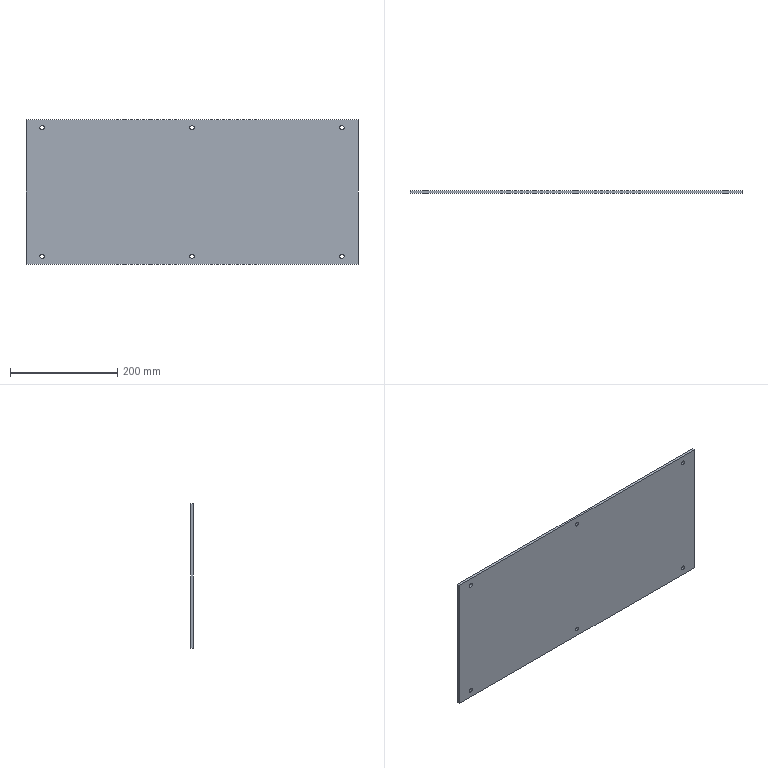Part | STEP file | OP10-003_front cover (R) | 1 solid | 18 faces | box 620 x 5 x 270 mm | volume 835492 mm3 | cylinder 12 | plane 6 | commonest cylinder face diameters 8 x12
STEP:
#1=CARTESIAN_POINT('',(0.,0.,0.));
#2=DIRECTION('',(0.,0.,1.));
#3=DIRECTION('',(1.,0.,0.));
#4=AXIS2_PLACEMENT_3D('',#1,#2,#3);
#5=CARTESIAN_POINT('',(280.,0.,124.));
#6=VERTEX_POINT('',#5);
#7=CARTESIAN_POINT('',(280.,5.,124.));
#8=VERTEX_POINT('',#7);
#9=CARTESIAN_POINT('',(280.,5.,124.));
#10=DIRECTION('',(0.,1.,0.));
#11=VECTOR('',#10,1.);
#12=LINE('',#9,#11);
#13=CARTESIAN_POINT('',(280.,5.,120.));
#14=DIRECTION('',(0.,1.,0.));
#15=DIRECTION('',(0.,0.,1.));
#16=AXIS2_PLACEMENT_3D('',#13,#14,#15);
#17=CYLINDRICAL_SURFACE('',#16,4.);
#18=CARTESIAN_POINT('',(6.283,0.));
#19=DIRECTION('',(0.,1.));
#20=VECTOR('',#19,1.);
#21=LINE('',#18,#20);
#22=(GEOMETRIC_REPRESENTATION_CONTEXT(2)PARAMETRIC_REPRESENTATION_CONTEXT()REPRESENTATION_CONTEXT('',''));
#23=DEFINITIONAL_REPRESENTATION('',(#21),#22);
#24=PCURVE('',#17,#23);
#25=CARTESIAN_POINT('',(280.,5.,120.));
#26=DIRECTION('',(0.,1.,0.));
#27=DIRECTION('',(0.,0.,1.));
#28=AXIS2_PLACEMENT_3D('',#25,#26,#27);
#29=CYLINDRICAL_SURFACE('',#28,4.);
#30=CARTESIAN_POINT('',(0.,0.));
#31=DIRECTION('',(0.,1.));
#32=VECTOR('',#31,1.);
#33=LINE('',#30,#32);
#34=(GEOMETRIC_REPRESENTATION_CONTEXT(2)PARAMETRIC_REPRESENTATION_CONTEXT()REPRESENTATION_CONTEXT('',''));
#35=DEFINITIONAL_REPRESENTATION('',(#33),#34);
#36=PCURVE('',#29,#35);
#37=SURFACE_CURVE('',#12,(#24,#36),.PCURVE_S1.);
#38=EDGE_CURVE('',#6,#8,#37,.T.);
#39=ORIENTED_EDGE('',*,*,#38,.T.);
#40=CARTESIAN_POINT('',(280.,5.,116.));
#41=VERTEX_POINT('',#40);
#42=CARTESIAN_POINT('',(280.,5.,120.));
#43=DIRECTION('',(0.,1.,0.));
#44=DIRECTION('',(0.,0.,1.));
#45=AXIS2_PLACEMENT_3D('',#42,#43,#44);
#46=CIRCLE('',#45,4.);
#47=CARTESIAN_POINT('',(0.,0.));
#48=DIRECTION('',(1.,0.));
#49=VECTOR('',#48,1.);
#50=LINE('',#47,#49);
#51=(GEOMETRIC_REPRESENTATION_CONTEXT(2)PARAMETRIC_REPRESENTATION_CONTEXT()REPRESENTATION_CONTEXT('',''));
#52=DEFINITIONAL_REPRESENTATION('',(#50),#51);
#53=PCURVE('',#17,#52);
#54=CARTESIAN_POINT('',(0.,5.,0.));
#55=DIRECTION('',(0.,-1.,0.));
#56=DIRECTION('',(0.,0.,-1.));
#57=AXIS2_PLACEMENT_3D('',#54,#55,#56);
#58=PLANE('',#57);
#59=CARTESIAN_POINT('',(-124.,280.));
#60=CARTESIAN_POINT('',(-124.,286.928));
#61=CARTESIAN_POINT('',(-118.,283.464));
#62=CARTESIAN_POINT('',(-112.,280.));
#63=CARTESIAN_POINT('',(-118.,276.536));
#64=CARTESIAN_POINT('',(-124.,273.072));
#65=CARTESIAN_POINT('',(-124.,280.));
#66=(BOUNDED_CURVE()B_SPLINE_CURVE(2,(#59,#60,#61,#62,#63,#64,#65),.UNSPECIFIED.,.T.,.F.)B_SPLINE_CURVE_WITH_KNOTS((1,2,2,2,2,1),(-2.094,0.,2.094,4.189,6.283,8.378),.UNSPECIFIED.)CURVE()GEOMETRIC_REPRESENTATION_ITEM()RATIONAL_B_SPLINE_CURVE((1.,0.5,1.,0.5,1.,0.5,1.))REPRESENTATION_ITEM(''));
#67=(GEOMETRIC_REPRESENTATION_CONTEXT(2)PARAMETRIC_REPRESENTATION_CONTEXT()REPRESENTATION_CONTEXT('',''));
#68=DEFINITIONAL_REPRESENTATION('',(#66),#67);
#69=PCURVE('',#58,#68);
#70=SURFACE_CURVE('',#46,(#53,#69),.PCURVE_S1.);
#71=EDGE_CURVE('',#41,#8,#70,.T.);
#72=ORIENTED_EDGE('',*,*,#71,.F.);
#73=CARTESIAN_POINT('',(280.,0.,116.));
#74=VERTEX_POINT('',#73);
#75=CARTESIAN_POINT('',(280.,5.,116.));
#76=DIRECTION('',(0.,1.,0.));
#77=VECTOR('',#76,1.);
#78=LINE('',#75,#77);
#79=CARTESIAN_POINT('',(3.142,0.));
#80=DIRECTION('',(0.,1.));
#81=VECTOR('',#80,1.);
#82=LINE('',#79,#81);
#83=(GEOMETRIC_REPRESENTATION_CONTEXT(2)PARAMETRIC_REPRESENTATION_CONTEXT()REPRESENTATION_CONTEXT('',''));
#84=DEFINITIONAL_REPRESENTATION('',(#82),#83);
#85=PCURVE('',#17,#84);
#86=CARTESIAN_POINT('',(3.142,0.));
#87=DIRECTION('',(0.,1.));
#88=VECTOR('',#87,1.);
#89=LINE('',#86,#88);
#90=(GEOMETRIC_REPRESENTATION_CONTEXT(2)PARAMETRIC_REPRESENTATION_CONTEXT()REPRESENTATION_CONTEXT('',''));
#91=DEFINITIONAL_REPRESENTATION('',(#89),#90);
#92=PCURVE('',#29,#91);
#93=SURFACE_CURVE('',#78,(#85,#92),.PCURVE_S1.);
#94=EDGE_CURVE('',#74,#41,#93,.T.);
#95=ORIENTED_EDGE('',*,*,#94,.F.);
#96=CARTESIAN_POINT('',(280.,0.,120.));
#97=DIRECTION('',(0.,-1.,0.));
#98=DIRECTION('',(0.,0.,-1.));
#99=AXIS2_PLACEMENT_3D('',#96,#97,#98);
#100=CIRCLE('',#99,4.);
#101=CARTESIAN_POINT('',(9.425,-5.));
#102=DIRECTION('',(-1.,0.));
#103=VECTOR('',#102,1.);
#104=LINE('',#101,#103);
#105=(GEOMETRIC_REPRESENTATION_CONTEXT(2)PARAMETRIC_REPRESENTATION_CONTEXT()REPRESENTATION_CONTEXT('',''));
#106=DEFINITIONAL_REPRESENTATION('',(#104),#105);
#107=PCURVE('',#17,#106);
#108=CARTESIAN_POINT('',(0.,0.,0.));
#109=DIRECTION('',(0.,-1.,0.));
#110=DIRECTION('',(0.,0.,-1.));
#111=AXIS2_PLACEMENT_3D('',#108,#109,#110);
#112=PLANE('',#111);
#113=CARTESIAN_POINT('',(-120.,280.));
#114=DIRECTION('',(1.,0.));
#115=AXIS2_PLACEMENT_2D('',#113,#114);
#116=CIRCLE('',#115,4.);
#117=(GEOMETRIC_REPRESENTATION_CONTEXT(2)PARAMETRIC_REPRESENTATION_CONTEXT()REPRESENTATION_CONTEXT('',''));
#118=DEFINITIONAL_REPRESENTATION('',(#116),#117);
#119=PCURVE('',#112,#118);
#120=SURFACE_CURVE('',#100,(#107,#119),.PCURVE_S1.);
#121=EDGE_CURVE('',#6,#74,#120,.T.);
#122=ORIENTED_EDGE('',*,*,#121,.F.);
#123=EDGE_LOOP('',(#39,#72,#95,#122));
#124=FACE_BOUND('',#123,.F.);
#125=ADVANCED_FACE('',(#124),#17,.F.);
#126=CARTESIAN_POINT('',(0.,0.,124.));
#127=VERTEX_POINT('',#126);
#128=CARTESIAN_POINT('',(0.,5.,124.));
#129=VERTEX_POINT('',#128);
#130=CARTESIAN_POINT('',(0.,5.,124.));
#131=DIRECTION('',(0.,1.,0.));
#132=VECTOR('',#131,1.);
#133=LINE('',#130,#132);
#134=CARTESIAN_POINT('',(0.,5.,120.));
#135=DIRECTION('',(0.,1.,0.));
#136=DIRECTION('',(0.,0.,1.));
#137=AXIS2_PLACEMENT_3D('',#134,#135,#136);
#138=CYLINDRICAL_SURFACE('',#137,4.);
#139=CARTESIAN_POINT('',(6.283,0.));
#140=DIRECTION('',(0.,1.));
#141=VECTOR('',#140,1.);
#142=LINE('',#139,#141);
#143=(GEOMETRIC_REPRESENTATION_CONTEXT(2)PARAMETRIC_REPRESENTATION_CONTEXT()REPRESENTATION_CONTEXT('',''));
#144=DEFINITIONAL_REPRESENTATION('',(#142),#143);
#145=PCURVE('',#138,#144);
#146=CARTESIAN_POINT('',(0.,5.,120.));
#147=DIRECTION('',(0.,1.,0.));
#148=DIRECTION('',(0.,0.,1.));
#149=AXIS2_PLACEMENT_3D('',#146,#147,#148);
#150=CYLINDRICAL_SURFACE('',#149,4.);
#151=CARTESIAN_POINT('',(0.,0.));
#152=DIRECTION('',(0.,1.));
#153=VECTOR('',#152,1.);
#154=LINE('',#151,#153);
#155=(GEOMETRIC_REPRESENTATION_CONTEXT(2)PARAMETRIC_REPRESENTATION_CONTEXT()REPRESENTATION_CONTEXT('',''));
#156=DEFINITIONAL_REPRESENTATION('',(#154),#155);
#157=PCURVE('',#150,#156);
#158=SURFACE_CURVE('',#133,(#145,#157),.PCURVE_S1.);
#159=EDGE_CURVE('',#127,#129,#158,.T.);
#160=ORIENTED_EDGE('',*,*,#159,.T.);
#161=CARTESIAN_POINT('',(0.,5.,116.));
#162=VERTEX_POINT('',#161);
#163=CARTESIAN_POINT('',(0.,5.,120.));
#164=DIRECTION('',(0.,1.,0.));
#165=DIRECTION('',(0.,0.,1.));
#166=AXIS2_PLACEMENT_3D('',#163,#164,#165);
#167=CIRCLE('',#166,4.);
#168=CARTESIAN_POINT('',(0.,0.));
#169=DIRECTION('',(1.,0.));
#170=VECTOR('',#169,1.);
#171=LINE('',#168,#170);
#172=(GEOMETRIC_REPRESENTATION_CONTEXT(2)PARAMETRIC_REPRESENTATION_CONTEXT()REPRESENTATION_CONTEXT('',''));
#173=DEFINITIONAL_REPRESENTATION('',(#171),#172);
#174=PCURVE('',#138,#173);
#175=CARTESIAN_POINT('',(-124.,0.));
#176=CARTESIAN_POINT('',(-124.,6.928));
#177=CARTESIAN_POINT('',(-118.,3.464));
#178=CARTESIAN_POINT('',(-112.,0.));
#179=CARTESIAN_POINT('',(-118.,-3.464));
#180=CARTESIAN_POINT('',(-124.,-6.928));
#181=CARTESIAN_POINT('',(-124.,0.));
#182=(BOUNDED_CURVE()B_SPLINE_CURVE(2,(#175,#176,#177,#178,#179,#180,#181),.UNSPECIFIED.,.T.,.F.)B_SPLINE_CURVE_WITH_KNOTS((1,2,2,2,2,1),(-2.094,0.,2.094,4.189,6.283,8.378),.UNSPECIFIED.)CURVE()GEOMETRIC_REPRESENTATION_ITEM()RATIONAL_B_SPLINE_CURVE((1.,0.5,1.,0.5,1.,0.5,1.))REPRESENTATION_ITEM(''));
#183=(GEOMETRIC_REPRESENTATION_CONTEXT(2)PARAMETRIC_REPRESENTATION_CONTEXT()REPRESENTATION_CONTEXT('',''));
#184=DEFINITIONAL_REPRESENTATION('',(#182),#183);
#185=PCURVE('',#58,#184);
#186=SURFACE_CURVE('',#167,(#174,#185),.PCURVE_S1.);
#187=EDGE_CURVE('',#162,#129,#186,.T.);
#188=ORIENTED_EDGE('',*,*,#187,.F.);
#189=CARTESIAN_POINT('',(0.,0.,116.));
#190=VERTEX_POINT('',#189);
#191=CARTESIAN_POINT('',(0.,5.,116.));
#192=DIRECTION('',(0.,1.,0.));
#193=VECTOR('',#192,1.);
#194=LINE('',#191,#193);
#195=CARTESIAN_POINT('',(3.142,0.));
#196=DIRECTION('',(0.,1.));
#197=VECTOR('',#196,1.);
#198=LINE('',#195,#197);
#199=(GEOMETRIC_REPRESENTATION_CONTEXT(2)PARAMETRIC_REPRESENTATION_CONTEXT()REPRESENTATION_CONTEXT('',''));
#200=DEFINITIONAL_REPRESENTATION('',(#198),#199);
#201=PCURVE('',#138,#200);
#202=CARTESIAN_POINT('',(3.142,0.));
#203=DIRECTION('',(0.,1.));
#204=VECTOR('',#203,1.);
#205=LINE('',#202,#204);
#206=(GEOMETRIC_REPRESENTATION_CONTEXT(2)PARAMETRIC_REPRESENTATION_CONTEXT()REPRESENTATION_CONTEXT('',''));
#207=DEFINITIONAL_REPRESENTATION('',(#205),#206);
#208=PCURVE('',#150,#207);
#209=SURFACE_CURVE('',#194,(#201,#208),.PCURVE_S1.);
#210=EDGE_CURVE('',#190,#162,#209,.T.);
#211=ORIENTED_EDGE('',*,*,#210,.F.);
#212=CARTESIAN_POINT('',(0.,0.,120.));
#213=DIRECTION('',(0.,-1.,0.));
#214=DIRECTION('',(0.,0.,-1.));
#215=AXIS2_PLACEMENT_3D('',#212,#213,#214);
#216=CIRCLE('',#215,4.);
#217=CARTESIAN_POINT('',(9.425,-5.));
#218=DIRECTION('',(-1.,0.));
#219=VECTOR('',#218,1.);
#220=LINE('',#217,#219);
#221=(GEOMETRIC_REPRESENTATION_CONTEXT(2)PARAMETRIC_REPRESENTATION_CONTEXT()REPRESENTATION_CONTEXT('',''));
#222=DEFINITIONAL_REPRESENTATION('',(#220),#221);
#223=PCURVE('',#138,#222);
#224=CARTESIAN_POINT('',(-120.,0.));
#225=DIRECTION('',(1.,0.));
#226=AXIS2_PLACEMENT_2D('',#224,#225);
#227=CIRCLE('',#226,4.);
#228=(GEOMETRIC_REPRESENTATION_CONTEXT(2)PARAMETRIC_REPRESENTATION_CONTEXT()REPRESENTATION_CONTEXT('',''));
#229=DEFINITIONAL_REPRESENTATION('',(#227),#228);
#230=PCURVE('',#112,#229);
#231=SURFACE_CURVE('',#216,(#223,#230),.PCURVE_S1.);
#232=EDGE_CURVE('',#127,#190,#231,.T.);
#233=ORIENTED_EDGE('',*,*,#232,.F.);
#234=EDGE_LOOP('',(#160,#188,#211,#233));
#235=FACE_BOUND('',#234,.F.);
#236=ADVANCED_FACE('',(#235),#138,.F.);
#237=CARTESIAN_POINT('',(-280.,0.,124.));
#238=VERTEX_POINT('',#237);
#239=CARTESIAN_POINT('',(-280.,5.,124.));
#240=VERTEX_POINT('',#239);
#241=CARTESIAN_POINT('',(-280.,5.,124.));
#242=DIRECTION('',(0.,1.,0.));
#243=VECTOR('',#242,1.);
#244=LINE('',#241,#243);
#245=CARTESIAN_POINT('',(-280.,5.,120.));
#246=DIRECTION('',(0.,1.,0.));
#247=DIRECTION('',(0.,0.,1.));
#248=AXIS2_PLACEMENT_3D('',#245,#246,#247);
#249=CYLINDRICAL_SURFACE('',#248,4.);
#250=CARTESIAN_POINT('',(6.283,0.));
#251=DIRECTION('',(0.,1.));
#252=VECTOR('',#251,1.);
#253=LINE('',#250,#252);
#254=(GEOMETRIC_REPRESENTATION_CONTEXT(2)PARAMETRIC_REPRESENTATION_CONTEXT()REPRESENTATION_CONTEXT('',''));
#255=DEFINITIONAL_REPRESENTATION('',(#253),#254);
#256=PCURVE('',#249,#255);
#257=CARTESIAN_POINT('',(-280.,5.,120.));
#258=DIRECTION('',(0.,1.,0.));
#259=DIRECTION('',(0.,0.,1.));
#260=AXIS2_PLACEMENT_3D('',#257,#258,#259);
#261=CYLINDRICAL_SURFACE('',#260,4.);
#262=CARTESIAN_POINT('',(0.,0.));
#263=DIRECTION('',(0.,1.));
#264=VECTOR('',#263,1.);
#265=LINE('',#262,#264);
#266=(GEOMETRIC_REPRESENTATION_CONTEXT(2)PARAMETRIC_REPRESENTATION_CONTEXT()REPRESENTATION_CONTEXT('',''));
#267=DEFINITIONAL_REPRESENTATION('',(#265),#266);
#268=PCURVE('',#261,#267);
#269=SURFACE_CURVE('',#244,(#256,#268),.PCURVE_S1.);
#270=EDGE_CURVE('',#238,#240,#269,.T.);
#271=ORIENTED_EDGE('',*,*,#270,.T.);
#272=CARTESIAN_POINT('',(-280.,5.,116.));
#273=VERTEX_POINT('',#272);
#274=CARTESIAN_POINT('',(-280.,5.,120.));
#275=DIRECTION('',(0.,1.,0.));
#276=DIRECTION('',(0.,0.,1.));
#277=AXIS2_PLACEMENT_3D('',#274,#275,#276);
#278=CIRCLE('',#277,4.);
#279=CARTESIAN_POINT('',(0.,0.));
#280=DIRECTION('',(1.,0.));
#281=VECTOR('',#280,1.);
#282=LINE('',#279,#281);
#283=(GEOMETRIC_REPRESENTATION_CONTEXT(2)PARAMETRIC_REPRESENTATION_CONTEXT()REPRESENTATION_CONTEXT('',''));
#284=DEFINITIONAL_REPRESENTATION('',(#282),#283);
#285=PCURVE('',#249,#284);
#286=CARTESIAN_POINT('',(-124.,-280.));
#287=CARTESIAN_POINT('',(-124.,-273.072));
#288=CARTESIAN_POINT('',(-118.,-276.536));
#289=CARTESIAN_POINT('',(-112.,-280.));
#290=CARTESIAN_POINT('',(-118.,-283.464));
#291=CARTESIAN_POINT('',(-124.,-286.928));
#292=CARTESIAN_POINT('',(-124.,-280.));
#293=(BOUNDED_CURVE()B_SPLINE_CURVE(2,(#286,#287,#288,#289,#290,#291,#292),.UNSPECIFIED.,.T.,.F.)B_SPLINE_CURVE_WITH_KNOTS((1,2,2,2,2,1),(-2.094,0.,2.094,4.189,6.283,8.378),.UNSPECIFIED.)CURVE()GEOMETRIC_REPRESENTATION_ITEM()RATIONAL_B_SPLINE_CURVE((1.,0.5,1.,0.5,1.,0.5,1.))REPRESENTATION_ITEM(''));
#294=(GEOMETRIC_REPRESENTATION_CONTEXT(2)PARAMETRIC_REPRESENTATION_CONTEXT()REPRESENTATION_CONTEXT('',''));
#295=DEFINITIONAL_REPRESENTATION('',(#293),#294);
#296=PCURVE('',#58,#295);
#297=SURFACE_CURVE('',#278,(#285,#296),.PCURVE_S1.);
#298=EDGE_CURVE('',#273,#240,#297,.T.);
#299=ORIENTED_EDGE('',*,*,#298,.F.);
#300=CARTESIAN_POINT('',(-280.,0.,116.));
#301=VERTEX_POINT('',#300);
#302=CARTESIAN_POINT('',(-280.,5.,116.));
#303=DIRECTION('',(0.,1.,0.));
#304=VECTOR('',#303,1.);
#305=LINE('',#302,#304);
#306=CARTESIAN_POINT('',(3.142,0.));
#307=DIRECTION('',(0.,1.));
#308=VECTOR('',#307,1.);
#309=LINE('',#306,#308);
#310=(GEOMETRIC_REPRESENTATION_CONTEXT(2)PARAMETRIC_REPRESENTATION_CONTEXT()REPRESENTATION_CONTEXT('',''));
#311=DEFINITIONAL_REPRESENTATION('',(#309),#310);
#312=PCURVE('',#249,#311);
#313=CARTESIAN_POINT('',(3.142,0.));
#314=DIRECTION('',(0.,1.));
#315=VECTOR('',#314,1.);
#316=LINE('',#313,#315);
#317=(GEOMETRIC_REPRESENTATION_CONTEXT(2)PARAMETRIC_REPRESENTATION_CONTEXT()REPRESENTATION_CONTEXT('',''));
#318=DEFINITIONAL_REPRESENTATION('',(#316),#317);
#319=PCURVE('',#261,#318);
#320=SURFACE_CURVE('',#305,(#312,#319),.PCURVE_S1.);
#321=EDGE_CURVE('',#301,#273,#320,.T.);
#322=ORIENTED_EDGE('',*,*,#321,.F.);
#323=CARTESIAN_POINT('',(-280.,0.,120.));
#324=DIRECTION('',(0.,-1.,0.));
#325=DIRECTION('',(0.,0.,-1.));
#326=AXIS2_PLACEMENT_3D('',#323,#324,#325);
#327=CIRCLE('',#326,4.);
#328=CARTESIAN_POINT('',(9.425,-5.));
#329=DIRECTION('',(-1.,0.));
#330=VECTOR('',#329,1.);
#331=LINE('',#328,#330);
#332=(GEOMETRIC_REPRESENTATION_CONTEXT(2)PARAMETRIC_REPRESENTATION_CONTEXT()REPRESENTATION_CONTEXT('',''));
#333=DEFINITIONAL_REPRESENTATION('',(#331),#332);
#334=PCURVE('',#249,#333);
#335=CARTESIAN_POINT('',(-120.,-280.));
#336=DIRECTION('',(1.,0.));
#337=AXIS2_PLACEMENT_2D('',#335,#336);
#338=CIRCLE('',#337,4.);
#339=(GEOMETRIC_REPRESENTATION_CONTEXT(2)PARAMETRIC_REPRESENTATION_CONTEXT()REPRESENTATION_CONTEXT('',''));
#340=DEFINITIONAL_REPRESENTATION('',(#338),#339);
#341=PCURVE('',#112,#340);
#342=SURFACE_CURVE('',#327,(#334,#341),.PCURVE_S1.);
#343=EDGE_CURVE('',#238,#301,#342,.T.);
#344=ORIENTED_EDGE('',*,*,#343,.F.);
#345=EDGE_LOOP('',(#271,#299,#322,#344));
#346=FACE_BOUND('',#345,.F.);
#347=ADVANCED_FACE('',(#346),#249,.F.);
#348=CARTESIAN_POINT('',(280.,0.,-116.));
#349=VERTEX_POINT('',#348);
#350=CARTESIAN_POINT('',(280.,5.,-116.));
#351=VERTEX_POINT('',#350);
#352=CARTESIAN_POINT('',(280.,5.,-116.));
#353=DIRECTION('',(0.,1.,0.));
#354=VECTOR('',#353,1.);
#355=LINE('',#352,#354);
#356=CARTESIAN_POINT('',(280.,5.,-120.));
#357=DIRECTION('',(0.,1.,0.));
#358=DIRECTION('',(0.,0.,1.));
#359=AXIS2_PLACEMENT_3D('',#356,#357,#358);
#360=CYLINDRICAL_SURFACE('',#359,4.);
#361=CARTESIAN_POINT('',(6.283,0.));
#362=DIRECTION('',(0.,1.));
#363=VECTOR('',#362,1.);
#364=LINE('',#361,#363);
#365=(GEOMETRIC_REPRESENTATION_CONTEXT(2)PARAMETRIC_REPRESENTATION_CONTEXT()REPRESENTATION_CONTEXT('',''));
#366=DEFINITIONAL_REPRESENTATION('',(#364),#365);
#367=PCURVE('',#360,#366);
#368=CARTESIAN_POINT('',(280.,5.,-120.));
#369=DIRECTION('',(0.,1.,0.));
#370=DIRECTION('',(0.,0.,1.));
#371=AXIS2_PLACEMENT_3D('',#368,#369,#370);
#372=CYLINDRICAL_SURFACE('',#371,4.);
#373=CARTESIAN_POINT('',(0.,0.));
#374=DIRECTION('',(0.,1.));
#375=VECTOR('',#374,1.);
#376=LINE('',#373,#375);
#377=(GEOMETRIC_REPRESENTATION_CONTEXT(2)PARAMETRIC_REPRESENTATION_CONTEXT()REPRESENTATION_CONTEXT('',''));
#378=DEFINITIONAL_REPRESENTATION('',(#376),#377);
#379=PCURVE('',#372,#378);
#380=SURFACE_CURVE('',#355,(#367,#379),.PCURVE_S1.);
#381=EDGE_CURVE('',#349,#351,#380,.T.);
#382=ORIENTED_EDGE('',*,*,#381,.T.);
#383=CARTESIAN_POINT('',(280.,5.,-124.));
#384=VERTEX_POINT('',#383);
#385=CARTESIAN_POINT('',(280.,5.,-120.));
#386=DIRECTION('',(0.,1.,0.));
#387=DIRECTION('',(0.,0.,1.));
#388=AXIS2_PLACEMENT_3D('',#385,#386,#387);
#389=CIRCLE('',#388,4.);
#390=CARTESIAN_POINT('',(0.,0.));
#391=DIRECTION('',(1.,0.));
#392=VECTOR('',#391,1.);
#393=LINE('',#390,#392);
#394=(GEOMETRIC_REPRESENTATION_CONTEXT(2)PARAMETRIC_REPRESENTATION_CONTEXT()REPRESENTATION_CONTEXT('',''));
#395=DEFINITIONAL_REPRESENTATION('',(#393),#394);
#396=PCURVE('',#360,#395);
#397=CARTESIAN_POINT('',(116.,280.));
#398=CARTESIAN_POINT('',(116.,286.928));
#399=CARTESIAN_POINT('',(122.,283.464));
#400=CARTESIAN_POINT('',(128.,280.));
#401=CARTESIAN_POINT('',(122.,276.536));
#402=CARTESIAN_POINT('',(116.,273.072));
#403=CARTESIAN_POINT('',(116.,280.));
#404=(BOUNDED_CURVE()B_SPLINE_CURVE(2,(#397,#398,#399,#400,#401,#402,#403),.UNSPECIFIED.,.T.,.F.)B_SPLINE_CURVE_WITH_KNOTS((1,2,2,2,2,1),(-2.094,0.,2.094,4.189,6.283,8.378),.UNSPECIFIED.)CURVE()GEOMETRIC_REPRESENTATION_ITEM()RATIONAL_B_SPLINE_CURVE((1.,0.5,1.,0.5,1.,0.5,1.))REPRESENTATION_ITEM(''));
#405=(GEOMETRIC_REPRESENTATION_CONTEXT(2)PARAMETRIC_REPRESENTATION_CONTEXT()REPRESENTATION_CONTEXT('',''));
#406=DEFINITIONAL_REPRESENTATION('',(#404),#405);
#407=PCURVE('',#58,#406);
#408=SURFACE_CURVE('',#389,(#396,#407),.PCURVE_S1.);
#409=EDGE_CURVE('',#384,#351,#408,.T.);
#410=ORIENTED_EDGE('',*,*,#409,.F.);
#411=CARTESIAN_POINT('',(280.,0.,-124.));
#412=VERTEX_POINT('',#411);
#413=CARTESIAN_POINT('',(280.,5.,-124.));
#414=DIRECTION('',(0.,1.,0.));
#415=VECTOR('',#414,1.);
#416=LINE('',#413,#415);
#417=CARTESIAN_POINT('',(3.142,0.));
#418=DIRECTION('',(0.,1.));
#419=VECTOR('',#418,1.);
#420=LINE('',#417,#419);
#421=(GEOMETRIC_REPRESENTATION_CONTEXT(2)PARAMETRIC_REPRESENTATION_CONTEXT()REPRESENTATION_CONTEXT('',''));
#422=DEFINITIONAL_REPRESENTATION('',(#420),#421);
#423=PCURVE('',#360,#422);
#424=CARTESIAN_POINT('',(3.142,0.));
#425=DIRECTION('',(0.,1.));
#426=VECTOR('',#425,1.);
#427=LINE('',#424,#426);
#428=(GEOMETRIC_REPRESENTATION_CONTEXT(2)PARAMETRIC_REPRESENTATION_CONTEXT()REPRESENTATION_CONTEXT('',''));
#429=DEFINITIONAL_REPRESENTATION('',(#427),#428);
#430=PCURVE('',#372,#429);
#431=SURFACE_CURVE('',#416,(#423,#430),.PCURVE_S1.);
#432=EDGE_CURVE('',#412,#384,#431,.T.);
#433=ORIENTED_EDGE('',*,*,#432,.F.);
#434=CARTESIAN_POINT('',(280.,0.,-120.));
#435=DIRECTION('',(0.,-1.,0.));
#436=DIRECTION('',(0.,0.,-1.));
#437=AXIS2_PLACEMENT_3D('',#434,#435,#436);
#438=CIRCLE('',#437,4.);
#439=CARTESIAN_POINT('',(9.425,-5.));
#440=DIRECTION('',(-1.,0.));
#441=VECTOR('',#440,1.);
#442=LINE('',#439,#441);
#443=(GEOMETRIC_REPRESENTATION_CONTEXT(2)PARAMETRIC_REPRESENTATION_CONTEXT()REPRESENTATION_CONTEXT('',''));
#444=DEFINITIONAL_REPRESENTATION('',(#442),#443);
#445=PCURVE('',#360,#444);
#446=CARTESIAN_POINT('',(120.,280.));
#447=DIRECTION('',(1.,0.));
#448=AXIS2_PLACEMENT_2D('',#446,#447);
#449=CIRCLE('',#448,4.);
#450=(GEOMETRIC_REPRESENTATION_CONTEXT(2)PARAMETRIC_REPRESENTATION_CONTEXT()REPRESENTATION_CONTEXT('',''));
#451=DEFINITIONAL_REPRESENTATION('',(#449),#450);
#452=PCURVE('',#112,#451);
#453=SURFACE_CURVE('',#438,(#445,#452),.PCURVE_S1.);
#454=EDGE_CURVE('',#349,#412,#453,.T.);
#455=ORIENTED_EDGE('',*,*,#454,.F.);
#456=EDGE_LOOP('',(#382,#410,#433,#455));
#457=FACE_BOUND('',#456,.F.);
#458=ADVANCED_FACE('',(#457),#360,.F.);
#459=CARTESIAN_POINT('',(0.,0.,-116.));
#460=VERTEX_POINT('',#459);
#461=CARTESIAN_POINT('',(0.,5.,-116.));
#462=VERTEX_POINT('',#461);
#463=CARTESIAN_POINT('',(0.,5.,-116.));
#464=DIRECTION('',(0.,1.,0.));
#465=VECTOR('',#464,1.);
#466=LINE('',#463,#465);
#467=CARTESIAN_POINT('',(0.,5.,-120.));
#468=DIRECTION('',(0.,1.,0.));
#469=DIRECTION('',(0.,0.,1.));
#470=AXIS2_PLACEMENT_3D('',#467,#468,#469);
#471=CYLINDRICAL_SURFACE('',#470,4.);
#472=CARTESIAN_POINT('',(6.283,0.));
#473=DIRECTION('',(0.,1.));
#474=VECTOR('',#473,1.);
#475=LINE('',#472,#474);
#476=(GEOMETRIC_REPRESENTATION_CONTEXT(2)PARAMETRIC_REPRESENTATION_CONTEXT()REPRESENTATION_CONTEXT('',''));
#477=DEFINITIONAL_REPRESENTATION('',(#475),#476);
#478=PCURVE('',#471,#477);
#479=CARTESIAN_POINT('',(0.,5.,-120.));
#480=DIRECTION('',(0.,1.,0.));
#481=DIRECTION('',(0.,0.,1.));
#482=AXIS2_PLACEMENT_3D('',#479,#480,#481);
#483=CYLINDRICAL_SURFACE('',#482,4.);
#484=CARTESIAN_POINT('',(0.,0.));
#485=DIRECTION('',(0.,1.));
#486=VECTOR('',#485,1.);
#487=LINE('',#484,#486);
#488=(GEOMETRIC_REPRESENTATION_CONTEXT(2)PARAMETRIC_REPRESENTATION_CONTEXT()REPRESENTATION_CONTEXT('',''));
#489=DEFINITIONAL_REPRESENTATION('',(#487),#488);
#490=PCURVE('',#483,#489);
#491=SURFACE_CURVE('',#466,(#478,#490),.PCURVE_S1.);
#492=EDGE_CURVE('',#460,#462,#491,.T.);
#493=ORIENTED_EDGE('',*,*,#492,.T.);
#494=CARTESIAN_POINT('',(0.,5.,-124.));
#495=VERTEX_POINT('',#494);
#496=CARTESIAN_POINT('',(0.,5.,-120.));
#497=DIRECTION('',(0.,1.,0.));
#498=DIRECTION('',(0.,0.,1.));
#499=AXIS2_PLACEMENT_3D('',#496,#497,#498);
#500=CIRCLE('',#499,4.);
#501=CARTESIAN_POINT('',(0.,0.));
#502=DIRECTION('',(1.,0.));
#503=VECTOR('',#502,1.);
#504=LINE('',#501,#503);
#505=(GEOMETRIC_REPRESENTATION_CONTEXT(2)PARAMETRIC_REPRESENTATION_CONTEXT()REPRESENTATION_CONTEXT('',''));
#506=DEFINITIONAL_REPRESENTATION('',(#504),#505);
#507=PCURVE('',#471,#506);
#508=CARTESIAN_POINT('',(116.,0.));
#509=CARTESIAN_POINT('',(116.,6.928));
#510=CARTESIAN_POINT('',(122.,3.464));
#511=CARTESIAN_POINT('',(128.,0.));
#512=CARTESIAN_POINT('',(122.,-3.464));
#513=CARTESIAN_POINT('',(116.,-6.928));
#514=CARTESIAN_POINT('',(116.,0.));
#515=(BOUNDED_CURVE()B_SPLINE_CURVE(2,(#508,#509,#510,#511,#512,#513,#514),.UNSPECIFIED.,.T.,.F.)B_SPLINE_CURVE_WITH_KNOTS((1,2,2,2,2,1),(-2.094,0.,2.094,4.189,6.283,8.378),.UNSPECIFIED.)CURVE()GEOMETRIC_REPRESENTATION_ITEM()RATIONAL_B_SPLINE_CURVE((1.,0.5,1.,0.5,1.,0.5,1.))REPRESENTATION_ITEM(''));
#516=(GEOMETRIC_REPRESENTATION_CONTEXT(2)PARAMETRIC_REPRESENTATION_CONTEXT()REPRESENTATION_CONTEXT('',''));
#517=DEFINITIONAL_REPRESENTATION('',(#515),#516);
#518=PCURVE('',#58,#517);
#519=SURFACE_CURVE('',#500,(#507,#518),.PCURVE_S1.);
#520=EDGE_CURVE('',#495,#462,#519,.T.);
#521=ORIENTED_EDGE('',*,*,#520,.F.);
#522=CARTESIAN_POINT('',(0.,0.,-124.));
#523=VERTEX_POINT('',#522);
#524=CARTESIAN_POINT('',(0.,5.,-124.));
#525=DIRECTION('',(0.,1.,0.));
#526=VECTOR('',#525,1.);
#527=LINE('',#524,#526);
#528=CARTESIAN_POINT('',(3.142,0.));
#529=DIRECTION('',(0.,1.));
#530=VECTOR('',#529,1.);
#531=LINE('',#528,#530);
#532=(GEOMETRIC_REPRESENTATION_CONTEXT(2)PARAMETRIC_REPRESENTATION_CONTEXT()REPRESENTATION_CONTEXT('',''));
#533=DEFINITIONAL_REPRESENTATION('',(#531),#532);
#534=PCURVE('',#471,#533);
#535=CARTESIAN_POINT('',(3.142,0.));
#536=DIRECTION('',(0.,1.));
#537=VECTOR('',#536,1.);
#538=LINE('',#535,#537);
#539=(GEOMETRIC_REPRESENTATION_CONTEXT(2)PARAMETRIC_REPRESENTATION_CONTEXT()REPRESENTATION_CONTEXT('',''));
#540=DEFINITIONAL_REPRESENTATION('',(#538),#539);
#541=PCURVE('',#483,#540);
#542=SURFACE_CURVE('',#527,(#534,#541),.PCURVE_S1.);
#543=EDGE_CURVE('',#523,#495,#542,.T.);
#544=ORIENTED_EDGE('',*,*,#543,.F.);
#545=CARTESIAN_POINT('',(0.,0.,-120.));
#546=DIRECTION('',(0.,-1.,0.));
#547=DIRECTION('',(0.,0.,-1.));
#548=AXIS2_PLACEMENT_3D('',#545,#546,#547);
#549=CIRCLE('',#548,4.);
#550=CARTESIAN_POINT('',(9.425,-5.));
#551=DIRECTION('',(-1.,0.));
#552=VECTOR('',#551,1.);
#553=LINE('',#550,#552);
#554=(GEOMETRIC_REPRESENTATION_CONTEXT(2)PARAMETRIC_REPRESENTATION_CONTEXT()REPRESENTATION_CONTEXT('',''));
#555=DEFINITIONAL_REPRESENTATION('',(#553),#554);
#556=PCURVE('',#471,#555);
#557=CARTESIAN_POINT('',(120.,0.));
#558=DIRECTION('',(1.,0.));
#559=AXIS2_PLACEMENT_2D('',#557,#558);
#560=CIRCLE('',#559,4.);
#561=(GEOMETRIC_REPRESENTATION_CONTEXT(2)PARAMETRIC_REPRESENTATION_CONTEXT()REPRESENTATION_CONTEXT('',''));
#562=DEFINITIONAL_REPRESENTATION('',(#560),#561);
#563=PCURVE('',#112,#562);
#564=SURFACE_CURVE('',#549,(#556,#563),.PCURVE_S1.);
#565=EDGE_CURVE('',#460,#523,#564,.T.);
#566=ORIENTED_EDGE('',*,*,#565,.F.);
#567=EDGE_LOOP('',(#493,#521,#544,#566));
#568=FACE_BOUND('',#567,.F.);
#569=ADVANCED_FACE('',(#568),#471,.F.);
#570=CARTESIAN_POINT('',(-280.,0.,-116.));
#571=VERTEX_POINT('',#570);
#572=CARTESIAN_POINT('',(-280.,5.,-116.));
#573=VERTEX_POINT('',#572);
#574=CARTESIAN_POINT('',(-280.,5.,-116.));
#575=DIRECTION('',(0.,1.,0.));
#576=VECTOR('',#575,1.);
#577=LINE('',#574,#576);
#578=CARTESIAN_POINT('',(-280.,5.,-120.));
#579=DIRECTION('',(0.,1.,0.));
#580=DIRECTION('',(0.,0.,1.));
#581=AXIS2_PLACEMENT_3D('',#578,#579,#580);
#582=CYLINDRICAL_SURFACE('',#581,4.);
#583=CARTESIAN_POINT('',(6.283,0.));
#584=DIRECTION('',(0.,1.));
#585=VECTOR('',#584,1.);
#586=LINE('',#583,#585);
#587=(GEOMETRIC_REPRESENTATION_CONTEXT(2)PARAMETRIC_REPRESENTATION_CONTEXT()REPRESENTATION_CONTEXT('',''));
#588=DEFINITIONAL_REPRESENTATION('',(#586),#587);
#589=PCURVE('',#582,#588);
#590=CARTESIAN_POINT('',(-280.,5.,-120.));
#591=DIRECTION('',(0.,1.,0.));
#592=DIRECTION('',(0.,0.,1.));
#593=AXIS2_PLACEMENT_3D('',#590,#591,#592);
#594=CYLINDRICAL_SURFACE('',#593,4.);
#595=CARTESIAN_POINT('',(0.,0.));
#596=DIRECTION('',(0.,1.));
#597=VECTOR('',#596,1.);
#598=LINE('',#595,#597);
#599=(GEOMETRIC_REPRESENTATION_CONTEXT(2)PARAMETRIC_REPRESENTATION_CONTEXT()REPRESENTATION_CONTEXT('',''));
#600=DEFINITIONAL_REPRESENTATION('',(#598),#599);
#601=PCURVE('',#594,#600);
#602=SURFACE_CURVE('',#577,(#589,#601),.PCURVE_S1.);
#603=EDGE_CURVE('',#571,#573,#602,.T.);
#604=ORIENTED_EDGE('',*,*,#603,.T.);
#605=CARTESIAN_POINT('',(-280.,5.,-124.));
#606=VERTEX_POINT('',#605);
#607=CARTESIAN_POINT('',(-280.,5.,-120.));
#608=DIRECTION('',(0.,1.,0.));
#609=DIRECTION('',(0.,0.,1.));
#610=AXIS2_PLACEMENT_3D('',#607,#608,#609);
#611=CIRCLE('',#610,4.);
#612=CARTESIAN_POINT('',(0.,0.));
#613=DIRECTION('',(1.,0.));
#614=VECTOR('',#613,1.);
#615=LINE('',#612,#614);
#616=(GEOMETRIC_REPRESENTATION_CONTEXT(2)PARAMETRIC_REPRESENTATION_CONTEXT()REPRESENTATION_CONTEXT('',''));
#617=DEFINITIONAL_REPRESENTATION('',(#615),#616);
#618=PCURVE('',#582,#617);
#619=CARTESIAN_POINT('',(116.,-280.));
#620=CARTESIAN_POINT('',(116.,-273.072));
#621=CARTESIAN_POINT('',(122.,-276.536));
#622=CARTESIAN_POINT('',(128.,-280.));
#623=CARTESIAN_POINT('',(122.,-283.464));
#624=CARTESIAN_POINT('',(116.,-286.928));
#625=CARTESIAN_POINT('',(116.,-280.));
#626=(BOUNDED_CURVE()B_SPLINE_CURVE(2,(#619,#620,#621,#622,#623,#624,#625),.UNSPECIFIED.,.T.,.F.)B_SPLINE_CURVE_WITH_KNOTS((1,2,2,2,2,1),(-2.094,0.,2.094,4.189,6.283,8.378),.UNSPECIFIED.)CURVE()GEOMETRIC_REPRESENTATION_ITEM()RATIONAL_B_SPLINE_CURVE((1.,0.5,1.,0.5,1.,0.5,1.))REPRESENTATION_ITEM(''));
#627=(GEOMETRIC_REPRESENTATION_CONTEXT(2)PARAMETRIC_REPRESENTATION_CONTEXT()REPRESENTATION_CONTEXT('',''));
#628=DEFINITIONAL_REPRESENTATION('',(#626),#627);
#629=PCURVE('',#58,#628);
#630=SURFACE_CURVE('',#611,(#618,#629),.PCURVE_S1.);
#631=EDGE_CURVE('',#606,#573,#630,.T.);
#632=ORIENTED_EDGE('',*,*,#631,.F.);
#633=CARTESIAN_POINT('',(-280.,0.,-124.));
#634=VERTEX_POINT('',#633);
#635=CARTESIAN_POINT('',(-280.,5.,-124.));
#636=DIRECTION('',(0.,1.,0.));
#637=VECTOR('',#636,1.);
#638=LINE('',#635,#637);
#639=CARTESIAN_POINT('',(3.142,0.));
#640=DIRECTION('',(0.,1.));
#641=VECTOR('',#640,1.);
#642=LINE('',#639,#641);
#643=(GEOMETRIC_REPRESENTATION_CONTEXT(2)PARAMETRIC_REPRESENTATION_CONTEXT()REPRESENTATION_CONTEXT('',''));
#644=DEFINITIONAL_REPRESENTATION('',(#642),#643);
#645=PCURVE('',#582,#644);
#646=CARTESIAN_POINT('',(3.142,0.));
#647=DIRECTION('',(0.,1.));
#648=VECTOR('',#647,1.);
#649=LINE('',#646,#648);
#650=(GEOMETRIC_REPRESENTATION_CONTEXT(2)PARAMETRIC_REPRESENTATION_CONTEXT()REPRESENTATION_CONTEXT('',''));
#651=DEFINITIONAL_REPRESENTATION('',(#649),#650);
#652=PCURVE('',#594,#651);
#653=SURFACE_CURVE('',#638,(#645,#652),.PCURVE_S1.);
#654=EDGE_CURVE('',#634,#606,#653,.T.);
#655=ORIENTED_EDGE('',*,*,#654,.F.);
#656=CARTESIAN_POINT('',(-280.,0.,-120.));
#657=DIRECTION('',(0.,-1.,0.));
#658=DIRECTION('',(0.,0.,-1.));
#659=AXIS2_PLACEMENT_3D('',#656,#657,#658);
#660=CIRCLE('',#659,4.);
#661=CARTESIAN_POINT('',(9.425,-5.));
#662=DIRECTION('',(-1.,0.));
#663=VECTOR('',#662,1.);
#664=LINE('',#661,#663);
#665=(GEOMETRIC_REPRESENTATION_CONTEXT(2)PARAMETRIC_REPRESENTATION_CONTEXT()REPRESENTATION_CONTEXT('',''));
#666=DEFINITIONAL_REPRESENTATION('',(#664),#665);
#667=PCURVE('',#582,#666);
#668=CARTESIAN_POINT('',(120.,-280.));
#669=DIRECTION('',(1.,0.));
#670=AXIS2_PLACEMENT_2D('',#668,#669);
#671=CIRCLE('',#670,4.);
#672=(GEOMETRIC_REPRESENTATION_CONTEXT(2)PARAMETRIC_REPRESENTATION_CONTEXT()REPRESENTATION_CONTEXT('',''));
#673=DEFINITIONAL_REPRESENTATION('',(#671),#672);
#674=PCURVE('',#112,#673);
#675=SURFACE_CURVE('',#660,(#667,#674),.PCURVE_S1.);
#676=EDGE_CURVE('',#571,#634,#675,.T.);
#677=ORIENTED_EDGE('',*,*,#676,.F.);
#678=EDGE_LOOP('',(#604,#632,#655,#677));
#679=FACE_BOUND('',#678,.F.);
#680=ADVANCED_FACE('',(#679),#582,.F.);
#681=CARTESIAN_POINT('',(310.,0.,135.));
#682=VERTEX_POINT('',#681);
#683=CARTESIAN_POINT('',(310.,0.,-135.));
#684=VERTEX_POINT('',#683);
#685=CARTESIAN_POINT('',(310.,0.,135.));
#686=DIRECTION('',(0.,0.,-1.));
#687=VECTOR('',#686,1.);
#688=LINE('',#685,#687);
#689=CARTESIAN_POINT('',(310.,5.,135.));
#690=DIRECTION('',(-1.,0.,0.));
#691=DIRECTION('',(0.,0.,1.));
#692=AXIS2_PLACEMENT_3D('',#689,#690,#691);
#693=PLANE('',#692);
#694=CARTESIAN_POINT('',(0.,-5.));
#695=DIRECTION('',(-1.,0.));
#696=VECTOR('',#695,1.);
#697=LINE('',#694,#696);
#698=(GEOMETRIC_REPRESENTATION_CONTEXT(2)PARAMETRIC_REPRESENTATION_CONTEXT()REPRESENTATION_CONTEXT('',''));
#699=DEFINITIONAL_REPRESENTATION('',(#697),#698);
#700=PCURVE('',#693,#699);
#701=CARTESIAN_POINT('',(-135.,310.));
#702=DIRECTION('',(1.,0.));
#703=VECTOR('',#702,1.);
#704=LINE('',#701,#703);
#705=(GEOMETRIC_REPRESENTATION_CONTEXT(2)PARAMETRIC_REPRESENTATION_CONTEXT()REPRESENTATION_CONTEXT('',''));
#706=DEFINITIONAL_REPRESENTATION('',(#704),#705);
#707=PCURVE('',#112,#706);
#708=SURFACE_CURVE('',#688,(#700,#707),.PCURVE_S1.);
#709=EDGE_CURVE('',#682,#684,#708,.T.);
#710=ORIENTED_EDGE('',*,*,#709,.T.);
#711=CARTESIAN_POINT('',(310.,5.,-135.));
#712=VERTEX_POINT('',#711);
#713=CARTESIAN_POINT('',(310.,5.,-135.));
#714=DIRECTION('',(0.,-1.,0.));
#715=VECTOR('',#714,1.);
#716=LINE('',#713,#715);
#717=CARTESIAN_POINT('',(-270.,0.));
#718=DIRECTION('',(0.,-1.));
#719=VECTOR('',#718,1.);
#720=LINE('',#717,#719);
#721=(GEOMETRIC_REPRESENTATION_CONTEXT(2)PARAMETRIC_REPRESENTATION_CONTEXT()REPRESENTATION_CONTEXT('',''));
#722=DEFINITIONAL_REPRESENTATION('',(#720),#721);
#723=PCURVE('',#693,#722);
#724=CARTESIAN_POINT('',(-310.,5.,-135.));
#725=DIRECTION('',(0.,0.,1.));
#726=DIRECTION('',(1.,0.,0.));
#727=AXIS2_PLACEMENT_3D('',#724,#725,#726);
#728=PLANE('',#727);
#729=CARTESIAN_POINT('',(620.,0.));
#730=DIRECTION('',(0.,-1.));
#731=VECTOR('',#730,1.);
#732=LINE('',#729,#731);
#733=(GEOMETRIC_REPRESENTATION_CONTEXT(2)PARAMETRIC_REPRESENTATION_CONTEXT()REPRESENTATION_CONTEXT('',''));
#734=DEFINITIONAL_REPRESENTATION('',(#732),#733);
#735=PCURVE('',#728,#734);
#736=SURFACE_CURVE('',#716,(#723,#735),.PCURVE_S1.);
#737=EDGE_CURVE('',#712,#684,#736,.T.);
#738=ORIENTED_EDGE('',*,*,#737,.F.);
#739=CARTESIAN_POINT('',(310.,5.,135.));
#740=VERTEX_POINT('',#739);
#741=CARTESIAN_POINT('',(310.,5.,135.));
#742=DIRECTION('',(0.,0.,-1.));
#743=VECTOR('',#742,1.);
#744=LINE('',#741,#743);
#745=CARTESIAN_POINT('',(0.,0.));
#746=DIRECTION('',(-1.,0.));
#747=VECTOR('',#746,1.);
#748=LINE('',#745,#747);
#749=(GEOMETRIC_REPRESENTATION_CONTEXT(2)PARAMETRIC_REPRESENTATION_CONTEXT()REPRESENTATION_CONTEXT('',''));
#750=DEFINITIONAL_REPRESENTATION('',(#748),#749);
#751=PCURVE('',#693,#750);
#752=CARTESIAN_POINT('',(-135.,310.));
#753=DIRECTION('',(1.,0.));
#754=VECTOR('',#753,1.);
#755=LINE('',#752,#754);
#756=(GEOMETRIC_REPRESENTATION_CONTEXT(2)PARAMETRIC_REPRESENTATION_CONTEXT()REPRESENTATION_CONTEXT('',''));
#757=DEFINITIONAL_REPRESENTATION('',(#755),#756);
#758=PCURVE('',#58,#757);
#759=SURFACE_CURVE('',#744,(#751,#758),.PCURVE_S1.);
#760=EDGE_CURVE('',#740,#712,#759,.T.);
#761=ORIENTED_EDGE('',*,*,#760,.F.);
#762=CARTESIAN_POINT('',(310.,5.,135.));
#763=DIRECTION('',(0.,-1.,0.));
#764=VECTOR('',#763,1.);
#765=LINE('',#762,#764);
#766=CARTESIAN_POINT('',(0.,0.));
#767=DIRECTION('',(0.,-1.));
#768=VECTOR('',#767,1.);
#769=LINE('',#766,#768);
#770=(GEOMETRIC_REPRESENTATION_CONTEXT(2)PARAMETRIC_REPRESENTATION_CONTEXT()REPRESENTATION_CONTEXT('',''));
#771=DEFINITIONAL_REPRESENTATION('',(#769),#770);
#772=PCURVE('',#693,#771);
#773=CARTESIAN_POINT('',(-310.,5.,135.));
#774=DIRECTION('',(0.,0.,-1.));
#775=DIRECTION('',(-1.,0.,0.));
#776=AXIS2_PLACEMENT_3D('',#773,#774,#775);
#777=PLANE('',#776);
#778=CARTESIAN_POINT('',(-620.,0.));
#779=DIRECTION('',(0.,-1.));
#780=VECTOR('',#779,1.);
#781=LINE('',#778,#780);
#782=(GEOMETRIC_REPRESENTATION_CONTEXT(2)PARAMETRIC_REPRESENTATION_CONTEXT()REPRESENTATION_CONTEXT('',''));
#783=DEFINITIONAL_REPRESENTATION('',(#781),#782);
#784=PCURVE('',#777,#783);
#785=SURFACE_CURVE('',#765,(#772,#784),.PCURVE_S1.);
#786=EDGE_CURVE('',#740,#682,#785,.T.);
#787=ORIENTED_EDGE('',*,*,#786,.T.);
#788=EDGE_LOOP('',(#710,#738,#761,#787));
#789=FACE_BOUND('',#788,.T.);
#790=ADVANCED_FACE('',(#789),#693,.F.);
#791=CARTESIAN_POINT('',(-310.,0.,-135.));
#792=VERTEX_POINT('',#791);
#793=CARTESIAN_POINT('',(-310.,0.,-135.));
#794=DIRECTION('',(-1.,0.,0.));
#795=VECTOR('',#794,1.);
#796=LINE('',#793,#795);
#797=CARTESIAN_POINT('',(0.,-5.));
#798=DIRECTION('',(-1.,0.));
#799=VECTOR('',#798,1.);
#800=LINE('',#797,#799);
#801=(GEOMETRIC_REPRESENTATION_CONTEXT(2)PARAMETRIC_REPRESENTATION_CONTEXT()REPRESENTATION_CONTEXT('',''));
#802=DEFINITIONAL_REPRESENTATION('',(#800),#801);
#803=PCURVE('',#728,#802);
#804=CARTESIAN_POINT('',(135.,-310.));
#805=DIRECTION('',(0.,-1.));
#806=VECTOR('',#805,1.);
#807=LINE('',#804,#806);
#808=(GEOMETRIC_REPRESENTATION_CONTEXT(2)PARAMETRIC_REPRESENTATION_CONTEXT()REPRESENTATION_CONTEXT('',''));
#809=DEFINITIONAL_REPRESENTATION('',(#807),#808);
#810=PCURVE('',#112,#809);
#811=SURFACE_CURVE('',#796,(#803,#810),.PCURVE_S1.);
#812=EDGE_CURVE('',#684,#792,#811,.T.);
#813=ORIENTED_EDGE('',*,*,#812,.T.);
#814=CARTESIAN_POINT('',(-310.,5.,-135.));
#815=VERTEX_POINT('',#814);
#816=CARTESIAN_POINT('',(-310.,5.,-135.));
#817=DIRECTION('',(0.,-1.,0.));
#818=VECTOR('',#817,1.);
#819=LINE('',#816,#818);
#820=CARTESIAN_POINT('',(0.,0.));
#821=DIRECTION('',(0.,-1.));
#822=VECTOR('',#821,1.);
#823=LINE('',#820,#822);
#824=(GEOMETRIC_REPRESENTATION_CONTEXT(2)PARAMETRIC_REPRESENTATION_CONTEXT()REPRESENTATION_CONTEXT('',''));
#825=DEFINITIONAL_REPRESENTATION('',(#823),#824);
#826=PCURVE('',#728,#825);
#827=CARTESIAN_POINT('',(-310.,5.,135.));
#828=DIRECTION('',(1.,0.,0.));
#829=DIRECTION('',(0.,0.,-1.));
#830=AXIS2_PLACEMENT_3D('',#827,#828,#829);
#831=PLANE('',#830);
#832=CARTESIAN_POINT('',(270.,0.));
#833=DIRECTION('',(0.,-1.));
#834=VECTOR('',#833,1.);
#835=LINE('',#832,#834);
#836=(GEOMETRIC_REPRESENTATION_CONTEXT(2)PARAMETRIC_REPRESENTATION_CONTEXT()REPRESENTATION_CONTEXT('',''));
#837=DEFINITIONAL_REPRESENTATION('',(#835),#836);
#838=PCURVE('',#831,#837);
#839=SURFACE_CURVE('',#819,(#826,#838),.PCURVE_S1.);
#840=EDGE_CURVE('',#815,#792,#839,.T.);
#841=ORIENTED_EDGE('',*,*,#840,.F.);
#842=CARTESIAN_POINT('',(-310.,5.,-135.));
#843=DIRECTION('',(-1.,0.,0.));
#844=VECTOR('',#843,1.);
#845=LINE('',#842,#844);
#846=CARTESIAN_POINT('',(0.,0.));
#847=DIRECTION('',(-1.,0.));
#848=VECTOR('',#847,1.);
#849=LINE('',#846,#848);
#850=(GEOMETRIC_REPRESENTATION_CONTEXT(2)PARAMETRIC_REPRESENTATION_CONTEXT()REPRESENTATION_CONTEXT('',''));
#851=DEFINITIONAL_REPRESENTATION('',(#849),#850);
#852=PCURVE('',#728,#851);
#853=CARTESIAN_POINT('',(135.,-310.));
#854=DIRECTION('',(0.,-1.));
#855=VECTOR('',#854,1.);
#856=LINE('',#853,#855);
#857=(GEOMETRIC_REPRESENTATION_CONTEXT(2)PARAMETRIC_REPRESENTATION_CONTEXT()REPRESENTATION_CONTEXT('',''));
#858=DEFINITIONAL_REPRESENTATION('',(#856),#857);
#859=PCURVE('',#58,#858);
#860=SURFACE_CURVE('',#845,(#852,#859),.PCURVE_S1.);
#861=EDGE_CURVE('',#712,#815,#860,.T.);
#862=ORIENTED_EDGE('',*,*,#861,.F.);
#863=ORIENTED_EDGE('',*,*,#737,.T.);
#864=EDGE_LOOP('',(#813,#841,#862,#863));
#865=FACE_BOUND('',#864,.T.);
#866=ADVANCED_FACE('',(#865),#728,.F.);
#867=CARTESIAN_POINT('',(-310.,0.,135.));
#868=VERTEX_POINT('',#867);
#869=CARTESIAN_POINT('',(-310.,0.,135.));
#870=DIRECTION('',(0.,0.,1.));
#871=VECTOR('',#870,1.);
#872=LINE('',#869,#871);
#873=CARTESIAN_POINT('',(0.,-5.));
#874=DIRECTION('',(-1.,0.));
#875=VECTOR('',#874,1.);
#876=LINE('',#873,#875);
#877=(GEOMETRIC_REPRESENTATION_CONTEXT(2)PARAMETRIC_REPRESENTATION_CONTEXT()REPRESENTATION_CONTEXT('',''));
#878=DEFINITIONAL_REPRESENTATION('',(#876),#877);
#879=PCURVE('',#831,#878);
#880=CARTESIAN_POINT('',(-135.,-310.));
#881=DIRECTION('',(-1.,0.));
#882=VECTOR('',#881,1.);
#883=LINE('',#880,#882);
#884=(GEOMETRIC_REPRESENTATION_CONTEXT(2)PARAMETRIC_REPRESENTATION_CONTEXT()REPRESENTATION_CONTEXT('',''));
#885=DEFINITIONAL_REPRESENTATION('',(#883),#884);
#886=PCURVE('',#112,#885);
#887=SURFACE_CURVE('',#872,(#879,#886),.PCURVE_S1.);
#888=EDGE_CURVE('',#792,#868,#887,.T.);
#889=ORIENTED_EDGE('',*,*,#888,.T.);
#890=CARTESIAN_POINT('',(-310.,5.,135.));
#891=VERTEX_POINT('',#890);
#892=CARTESIAN_POINT('',(-310.,5.,135.));
#893=DIRECTION('',(0.,-1.,0.));
#894=VECTOR('',#893,1.);
#895=LINE('',#892,#894);
#896=CARTESIAN_POINT('',(0.,0.));
#897=DIRECTION('',(0.,-1.));
#898=VECTOR('',#897,1.);
#899=LINE('',#896,#898);
#900=(GEOMETRIC_REPRESENTATION_CONTEXT(2)PARAMETRIC_REPRESENTATION_CONTEXT()REPRESENTATION_CONTEXT('',''));
#901=DEFINITIONAL_REPRESENTATION('',(#899),#900);
#902=PCURVE('',#831,#901);
#903=CARTESIAN_POINT('',(0.,0.));
#904=DIRECTION('',(0.,-1.));
#905=VECTOR('',#904,1.);
#906=LINE('',#903,#905);
#907=(GEOMETRIC_REPRESENTATION_CONTEXT(2)PARAMETRIC_REPRESENTATION_CONTEXT()REPRESENTATION_CONTEXT('',''));
#908=DEFINITIONAL_REPRESENTATION('',(#906),#907);
#909=PCURVE('',#777,#908);
#910=SURFACE_CURVE('',#895,(#902,#909),.PCURVE_S1.);
#911=EDGE_CURVE('',#891,#868,#910,.T.);
#912=ORIENTED_EDGE('',*,*,#911,.F.);
#913=CARTESIAN_POINT('',(-310.,5.,135.));
#914=DIRECTION('',(0.,0.,1.));
#915=VECTOR('',#914,1.);
#916=LINE('',#913,#915);
#917=CARTESIAN_POINT('',(0.,0.));
#918=DIRECTION('',(-1.,0.));
#919=VECTOR('',#918,1.);
#920=LINE('',#917,#919);
#921=(GEOMETRIC_REPRESENTATION_CONTEXT(2)PARAMETRIC_REPRESENTATION_CONTEXT()REPRESENTATION_CONTEXT('',''));
#922=DEFINITIONAL_REPRESENTATION('',(#920),#921);
#923=PCURVE('',#831,#922);
#924=CARTESIAN_POINT('',(-135.,-310.));
#925=DIRECTION('',(-1.,0.));
#926=VECTOR('',#925,1.);
#927=LINE('',#924,#926);
#928=(GEOMETRIC_REPRESENTATION_CONTEXT(2)PARAMETRIC_REPRESENTATION_CONTEXT()REPRESENTATION_CONTEXT('',''));
#929=DEFINITIONAL_REPRESENTATION('',(#927),#928);
#930=PCURVE('',#58,#929);
#931=SURFACE_CURVE('',#916,(#923,#930),.PCURVE_S1.);
#932=EDGE_CURVE('',#815,#891,#931,.T.);
#933=ORIENTED_EDGE('',*,*,#932,.F.);
#934=ORIENTED_EDGE('',*,*,#840,.T.);
#935=EDGE_LOOP('',(#889,#912,#933,#934));
#936=FACE_BOUND('',#935,.T.);
#937=ADVANCED_FACE('',(#936),#831,.F.);
#938=CARTESIAN_POINT('',(-310.,0.,135.));
#939=DIRECTION('',(1.,0.,0.));
#940=VECTOR('',#939,1.);
#941=LINE('',#938,#940);
#942=CARTESIAN_POINT('',(0.,-5.));
#943=DIRECTION('',(-1.,0.));
#944=VECTOR('',#943,1.);
#945=LINE('',#942,#944);
#946=(GEOMETRIC_REPRESENTATION_CONTEXT(2)PARAMETRIC_REPRESENTATION_CONTEXT()REPRESENTATION_CONTEXT('',''));
#947=DEFINITIONAL_REPRESENTATION('',(#945),#946);
#948=PCURVE('',#777,#947);
#949=CARTESIAN_POINT('',(-135.,-310.));
#950=DIRECTION('',(0.,1.));
#951=VECTOR('',#950,1.);
#952=LINE('',#949,#951);
#953=(GEOMETRIC_REPRESENTATION_CONTEXT(2)PARAMETRIC_REPRESENTATION_CONTEXT()REPRESENTATION_CONTEXT('',''));
#954=DEFINITIONAL_REPRESENTATION('',(#952),#953);
#955=PCURVE('',#112,#954);
#956=SURFACE_CURVE('',#941,(#948,#955),.PCURVE_S1.);
#957=EDGE_CURVE('',#868,#682,#956,.T.);
#958=ORIENTED_EDGE('',*,*,#957,.T.);
#959=ORIENTED_EDGE('',*,*,#786,.F.);
#960=CARTESIAN_POINT('',(-310.,5.,135.));
#961=DIRECTION('',(1.,0.,0.));
#962=VECTOR('',#961,1.);
#963=LINE('',#960,#962);
#964=CARTESIAN_POINT('',(0.,0.));
#965=DIRECTION('',(-1.,0.));
#966=VECTOR('',#965,1.);
#967=LINE('',#964,#966);
#968=(GEOMETRIC_REPRESENTATION_CONTEXT(2)PARAMETRIC_REPRESENTATION_CONTEXT()REPRESENTATION_CONTEXT('',''));
#969=DEFINITIONAL_REPRESENTATION('',(#967),#968);
#970=PCURVE('',#777,#969);
#971=CARTESIAN_POINT('',(-135.,-310.));
#972=DIRECTION('',(0.,1.));
#973=VECTOR('',#972,1.);
#974=LINE('',#971,#973);
#975=(GEOMETRIC_REPRESENTATION_CONTEXT(2)PARAMETRIC_REPRESENTATION_CONTEXT()REPRESENTATION_CONTEXT('',''));
#976=DEFINITIONAL_REPRESENTATION('',(#974),#975);
#977=PCURVE('',#58,#976);
#978=SURFACE_CURVE('',#963,(#970,#977),.PCURVE_S1.);
#979=EDGE_CURVE('',#891,#740,#978,.T.);
#980=ORIENTED_EDGE('',*,*,#979,.F.);
#981=ORIENTED_EDGE('',*,*,#911,.T.);
#982=EDGE_LOOP('',(#958,#959,#980,#981));
#983=FACE_BOUND('',#982,.T.);
#984=ADVANCED_FACE('',(#983),#777,.F.);
#985=CARTESIAN_POINT('',(0.,5.,-120.));
#986=DIRECTION('',(0.,1.,0.));
#987=DIRECTION('',(0.,0.,1.));
#988=AXIS2_PLACEMENT_3D('',#985,#986,#987);
#989=CIRCLE('',#988,4.);
#990=CARTESIAN_POINT('',(116.,0.));
#991=CARTESIAN_POINT('',(116.,6.928));
#992=CARTESIAN_POINT('',(122.,3.464));
#993=CARTESIAN_POINT('',(128.,0.));
#994=CARTESIAN_POINT('',(122.,-3.464));
#995=CARTESIAN_POINT('',(116.,-6.928));
#996=CARTESIAN_POINT('',(116.,0.));
#997=(BOUNDED_CURVE()B_SPLINE_CURVE(2,(#990,#991,#992,#993,#994,#995,#996),.UNSPECIFIED.,.T.,.F.)B_SPLINE_CURVE_WITH_KNOTS((1,2,2,2,2,1),(-2.094,0.,2.094,4.189,6.283,8.378),.UNSPECIFIED.)CURVE()GEOMETRIC_REPRESENTATION_ITEM()RATIONAL_B_SPLINE_CURVE((1.,0.5,1.,0.5,1.,0.5,1.))REPRESENTATION_ITEM(''));
#998=(GEOMETRIC_REPRESENTATION_CONTEXT(2)PARAMETRIC_REPRESENTATION_CONTEXT()REPRESENTATION_CONTEXT('',''));
#999=DEFINITIONAL_REPRESENTATION('',(#997),#998);
#1000=PCURVE('',#58,#999);
#1001=CARTESIAN_POINT('',(0.,0.));
#1002=DIRECTION('',(1.,0.));
#1003=VECTOR('',#1002,1.);
#1004=LINE('',#1001,#1003);
#1005=(GEOMETRIC_REPRESENTATION_CONTEXT(2)PARAMETRIC_REPRESENTATION_CONTEXT()REPRESENTATION_CONTEXT('',''));
#1006=DEFINITIONAL_REPRESENTATION('',(#1004),#1005);
#1007=PCURVE('',#483,#1006);
#1008=SURFACE_CURVE('',#989,(#1000,#1007),.PCURVE_S1.);
#1009=EDGE_CURVE('',#462,#495,#1008,.T.);
#1010=ORIENTED_EDGE('',*,*,#1009,.F.);
#1011=ORIENTED_EDGE('',*,*,#520,.F.);
#1012=EDGE_LOOP('',(#1010,#1011));
#1013=FACE_BOUND('',#1012,.T.);
#1014=CARTESIAN_POINT('',(-280.,5.,-120.));
#1015=DIRECTION('',(0.,1.,0.));
#1016=DIRECTION('',(0.,0.,1.));
#1017=AXIS2_PLACEMENT_3D('',#1014,#1015,#1016);
#1018=CIRCLE('',#1017,4.);
#1019=CARTESIAN_POINT('',(116.,-280.));
#1020=CARTESIAN_POINT('',(116.,-273.072));
#1021=CARTESIAN_POINT('',(122.,-276.536));
#1022=CARTESIAN_POINT('',(128.,-280.));
#1023=CARTESIAN_POINT('',(122.,-283.464));
#1024=CARTESIAN_POINT('',(116.,-286.928));
#1025=CARTESIAN_POINT('',(116.,-280.));
#1026=(BOUNDED_CURVE()B_SPLINE_CURVE(2,(#1019,#1020,#1021,#1022,#1023,#1024,#1025),.UNSPECIFIED.,.T.,.F.)B_SPLINE_CURVE_WITH_KNOTS((1,2,2,2,2,1),(-2.094,0.,2.094,4.189,6.283,8.378),.UNSPECIFIED.)CURVE()GEOMETRIC_REPRESENTATION_ITEM()RATIONAL_B_SPLINE_CURVE((1.,0.5,1.,0.5,1.,0.5,1.))REPRESENTATION_ITEM(''));
#1027=(GEOMETRIC_REPRESENTATION_CONTEXT(2)PARAMETRIC_REPRESENTATION_CONTEXT()REPRESENTATION_CONTEXT('',''));
#1028=DEFINITIONAL_REPRESENTATION('',(#1026),#1027);
#1029=PCURVE('',#58,#1028);
#1030=CARTESIAN_POINT('',(0.,0.));
#1031=DIRECTION('',(1.,0.));
#1032=VECTOR('',#1031,1.);
#1033=LINE('',#1030,#1032);
#1034=(GEOMETRIC_REPRESENTATION_CONTEXT(2)PARAMETRIC_REPRESENTATION_CONTEXT()REPRESENTATION_CONTEXT('',''));
#1035=DEFINITIONAL_REPRESENTATION('',(#1033),#1034);
#1036=PCURVE('',#594,#1035);
#1037=SURFACE_CURVE('',#1018,(#1029,#1036),.PCURVE_S1.);
#1038=EDGE_CURVE('',#573,#606,#1037,.T.);
#1039=ORIENTED_EDGE('',*,*,#1038,.F.);
#1040=ORIENTED_EDGE('',*,*,#631,.F.);
#1041=EDGE_LOOP('',(#1039,#1040));
#1042=FACE_BOUND('',#1041,.T.);
#1043=ORIENTED_EDGE('',*,*,#760,.T.);
#1044=ORIENTED_EDGE('',*,*,#861,.T.);
#1045=ORIENTED_EDGE('',*,*,#932,.T.);
#1046=ORIENTED_EDGE('',*,*,#979,.T.);
#1047=EDGE_LOOP('',(#1043,#1044,#1045,#1046));
#1048=FACE_BOUND('',#1047,.T.);
#1049=CARTESIAN_POINT('',(280.,5.,-120.));
#1050=DIRECTION('',(0.,1.,0.));
#1051=DIRECTION('',(0.,0.,1.));
#1052=AXIS2_PLACEMENT_3D('',#1049,#1050,#1051);
#1053=CIRCLE('',#1052,4.);
#1054=CARTESIAN_POINT('',(116.,280.));
#1055=CARTESIAN_POINT('',(116.,286.928));
#1056=CARTESIAN_POINT('',(122.,283.464));
#1057=CARTESIAN_POINT('',(128.,280.));
#1058=CARTESIAN_POINT('',(122.,276.536));
#1059=CARTESIAN_POINT('',(116.,273.072));
#1060=CARTESIAN_POINT('',(116.,280.));
#1061=(BOUNDED_CURVE()B_SPLINE_CURVE(2,(#1054,#1055,#1056,#1057,#1058,#1059,#1060),.UNSPECIFIED.,.T.,.F.)B_SPLINE_CURVE_WITH_KNOTS((1,2,2,2,2,1),(-2.094,0.,2.094,4.189,6.283,8.378),.UNSPECIFIED.)CURVE()GEOMETRIC_REPRESENTATION_ITEM()RATIONAL_B_SPLINE_CURVE((1.,0.5,1.,0.5,1.,0.5,1.))REPRESENTATION_ITEM(''));
#1062=(GEOMETRIC_REPRESENTATION_CONTEXT(2)PARAMETRIC_REPRESENTATION_CONTEXT()REPRESENTATION_CONTEXT('',''));
#1063=DEFINITIONAL_REPRESENTATION('',(#1061),#1062);
#1064=PCURVE('',#58,#1063);
#1065=CARTESIAN_POINT('',(0.,0.));
#1066=DIRECTION('',(1.,0.));
#1067=VECTOR('',#1066,1.);
#1068=LINE('',#1065,#1067);
#1069=(GEOMETRIC_REPRESENTATION_CONTEXT(2)PARAMETRIC_REPRESENTATION_CONTEXT()REPRESENTATION_CONTEXT('',''));
#1070=DEFINITIONAL_REPRESENTATION('',(#1068),#1069);
#1071=PCURVE('',#372,#1070);
#1072=SURFACE_CURVE('',#1053,(#1064,#1071),.PCURVE_S1.);
#1073=EDGE_CURVE('',#351,#384,#1072,.T.);
#1074=ORIENTED_EDGE('',*,*,#1073,.F.);
#1075=ORIENTED_EDGE('',*,*,#409,.F.);
#1076=EDGE_LOOP('',(#1074,#1075));
#1077=FACE_BOUND('',#1076,.T.);
#1078=CARTESIAN_POINT('',(-280.,5.,120.));
#1079=DIRECTION('',(0.,1.,0.));
#1080=DIRECTION('',(0.,0.,1.));
#1081=AXIS2_PLACEMENT_3D('',#1078,#1079,#1080);
#1082=CIRCLE('',#1081,4.);
#1083=CARTESIAN_POINT('',(-124.,-280.));
#1084=CARTESIAN_POINT('',(-124.,-273.072));
#1085=CARTESIAN_POINT('',(-118.,-276.536));
#1086=CARTESIAN_POINT('',(-112.,-280.));
#1087=CARTESIAN_POINT('',(-118.,-283.464));
#1088=CARTESIAN_POINT('',(-124.,-286.928));
#1089=CARTESIAN_POINT('',(-124.,-280.));
#1090=(BOUNDED_CURVE()B_SPLINE_CURVE(2,(#1083,#1084,#1085,#1086,#1087,#1088,#1089),.UNSPECIFIED.,.T.,.F.)B_SPLINE_CURVE_WITH_KNOTS((1,2,2,2,2,1),(-2.094,0.,2.094,4.189,6.283,8.378),.UNSPECIFIED.)CURVE()GEOMETRIC_REPRESENTATION_ITEM()RATIONAL_B_SPLINE_CURVE((1.,0.5,1.,0.5,1.,0.5,1.))REPRESENTATION_ITEM(''));
#1091=(GEOMETRIC_REPRESENTATION_CONTEXT(2)PARAMETRIC_REPRESENTATION_CONTEXT()REPRESENTATION_CONTEXT('',''));
#1092=DEFINITIONAL_REPRESENTATION('',(#1090),#1091);
#1093=PCURVE('',#58,#1092);
#1094=CARTESIAN_POINT('',(0.,0.));
#1095=DIRECTION('',(1.,0.));
#1096=VECTOR('',#1095,1.);
#1097=LINE('',#1094,#1096);
#1098=(GEOMETRIC_REPRESENTATION_CONTEXT(2)PARAMETRIC_REPRESENTATION_CONTEXT()REPRESENTATION_CONTEXT('',''));
#1099=DEFINITIONAL_REPRESENTATION('',(#1097),#1098);
#1100=PCURVE('',#261,#1099);
#1101=SURFACE_CURVE('',#1082,(#1093,#1100),.PCURVE_S1.);
#1102=EDGE_CURVE('',#240,#273,#1101,.T.);
#1103=ORIENTED_EDGE('',*,*,#1102,.F.);
#1104=ORIENTED_EDGE('',*,*,#298,.F.);
#1105=EDGE_LOOP('',(#1103,#1104));
#1106=FACE_BOUND('',#1105,.T.);
#1107=CARTESIAN_POINT('',(0.,5.,120.));
#1108=DIRECTION('',(0.,1.,0.));
#1109=DIRECTION('',(0.,0.,1.));
#1110=AXIS2_PLACEMENT_3D('',#1107,#1108,#1109);
#1111=CIRCLE('',#1110,4.);
#1112=CARTESIAN_POINT('',(-124.,0.));
#1113=CARTESIAN_POINT('',(-124.,6.928));
#1114=CARTESIAN_POINT('',(-118.,3.464));
#1115=CARTESIAN_POINT('',(-112.,0.));
#1116=CARTESIAN_POINT('',(-118.,-3.464));
#1117=CARTESIAN_POINT('',(-124.,-6.928));
#1118=CARTESIAN_POINT('',(-124.,0.));
#1119=(BOUNDED_CURVE()B_SPLINE_CURVE(2,(#1112,#1113,#1114,#1115,#1116,#1117,#1118),.UNSPECIFIED.,.T.,.F.)B_SPLINE_CURVE_WITH_KNOTS((1,2,2,2,2,1),(-2.094,0.,2.094,4.189,6.283,8.378),.UNSPECIFIED.)CURVE()GEOMETRIC_REPRESENTATION_ITEM()RATIONAL_B_SPLINE_CURVE((1.,0.5,1.,0.5,1.,0.5,1.))REPRESENTATION_ITEM(''));
#1120=(GEOMETRIC_REPRESENTATION_CONTEXT(2)PARAMETRIC_REPRESENTATION_CONTEXT()REPRESENTATION_CONTEXT('',''));
#1121=DEFINITIONAL_REPRESENTATION('',(#1119),#1120);
#1122=PCURVE('',#58,#1121);
#1123=CARTESIAN_POINT('',(0.,0.));
#1124=DIRECTION('',(1.,0.));
#1125=VECTOR('',#1124,1.);
#1126=LINE('',#1123,#1125);
#1127=(GEOMETRIC_REPRESENTATION_CONTEXT(2)PARAMETRIC_REPRESENTATION_CONTEXT()REPRESENTATION_CONTEXT('',''));
#1128=DEFINITIONAL_REPRESENTATION('',(#1126),#1127);
#1129=PCURVE('',#150,#1128);
#1130=SURFACE_CURVE('',#1111,(#1122,#1129),.PCURVE_S1.);
#1131=EDGE_CURVE('',#129,#162,#1130,.T.);
#1132=ORIENTED_EDGE('',*,*,#1131,.F.);
#1133=ORIENTED_EDGE('',*,*,#187,.F.);
#1134=EDGE_LOOP('',(#1132,#1133));
#1135=FACE_BOUND('',#1134,.T.);
#1136=CARTESIAN_POINT('',(280.,5.,120.));
#1137=DIRECTION('',(0.,1.,0.));
#1138=DIRECTION('',(0.,0.,1.));
#1139=AXIS2_PLACEMENT_3D('',#1136,#1137,#1138);
#1140=CIRCLE('',#1139,4.);
#1141=CARTESIAN_POINT('',(-124.,280.));
#1142=CARTESIAN_POINT('',(-124.,286.928));
#1143=CARTESIAN_POINT('',(-118.,283.464));
#1144=CARTESIAN_POINT('',(-112.,280.));
#1145=CARTESIAN_POINT('',(-118.,276.536));
#1146=CARTESIAN_POINT('',(-124.,273.072));
#1147=CARTESIAN_POINT('',(-124.,280.));
#1148=(BOUNDED_CURVE()B_SPLINE_CURVE(2,(#1141,#1142,#1143,#1144,#1145,#1146,#1147),.UNSPECIFIED.,.T.,.F.)B_SPLINE_CURVE_WITH_KNOTS((1,2,2,2,2,1),(-2.094,0.,2.094,4.189,6.283,8.378),.UNSPECIFIED.)CURVE()GEOMETRIC_REPRESENTATION_ITEM()RATIONAL_B_SPLINE_CURVE((1.,0.5,1.,0.5,1.,0.5,1.))REPRESENTATION_ITEM(''));
#1149=(GEOMETRIC_REPRESENTATION_CONTEXT(2)PARAMETRIC_REPRESENTATION_CONTEXT()REPRESENTATION_CONTEXT('',''));
#1150=DEFINITIONAL_REPRESENTATION('',(#1148),#1149);
#1151=PCURVE('',#58,#1150);
#1152=CARTESIAN_POINT('',(0.,0.));
#1153=DIRECTION('',(1.,0.));
#1154=VECTOR('',#1153,1.);
#1155=LINE('',#1152,#1154);
#1156=(GEOMETRIC_REPRESENTATION_CONTEXT(2)PARAMETRIC_REPRESENTATION_CONTEXT()REPRESENTATION_CONTEXT('',''));
#1157=DEFINITIONAL_REPRESENTATION('',(#1155),#1156);
#1158=PCURVE('',#29,#1157);
#1159=SURFACE_CURVE('',#1140,(#1151,#1158),.PCURVE_S1.);
#1160=EDGE_CURVE('',#8,#41,#1159,.T.);
#1161=ORIENTED_EDGE('',*,*,#1160,.F.);
#1162=ORIENTED_EDGE('',*,*,#71,.F.);
#1163=EDGE_LOOP('',(#1161,#1162));
#1164=FACE_BOUND('',#1163,.T.);
#1165=ADVANCED_FACE('',(#1013,#1042,#1048,#1077,#1106,#1135,#1164),#58,.F.);
#1166=ORIENTED_EDGE('',*,*,#565,.F.);
#1167=CARTESIAN_POINT('',(0.,0.,-120.));
#1168=DIRECTION('',(0.,-1.,0.));
#1169=DIRECTION('',(0.,0.,-1.));
#1170=AXIS2_PLACEMENT_3D('',#1167,#1168,#1169);
#1171=CIRCLE('',#1170,4.);
#1172=CARTESIAN_POINT('',(120.,0.));
#1173=DIRECTION('',(1.,0.));
#1174=AXIS2_PLACEMENT_2D('',#1172,#1173);
#1175=CIRCLE('',#1174,4.);
#1176=(GEOMETRIC_REPRESENTATION_CONTEXT(2)PARAMETRIC_REPRESENTATION_CONTEXT()REPRESENTATION_CONTEXT('',''));
#1177=DEFINITIONAL_REPRESENTATION('',(#1175),#1176);
#1178=PCURVE('',#112,#1177);
#1179=CARTESIAN_POINT('',(3.142,-5.));
#1180=DIRECTION('',(-1.,0.));
#1181=VECTOR('',#1180,1.);
#1182=LINE('',#1179,#1181);
#1183=(GEOMETRIC_REPRESENTATION_CONTEXT(2)PARAMETRIC_REPRESENTATION_CONTEXT()REPRESENTATION_CONTEXT('',''));
#1184=DEFINITIONAL_REPRESENTATION('',(#1182),#1183);
#1185=PCURVE('',#483,#1184);
#1186=SURFACE_CURVE('',#1171,(#1178,#1185),.PCURVE_S1.);
#1187=EDGE_CURVE('',#523,#460,#1186,.T.);
#1188=ORIENTED_EDGE('',*,*,#1187,.F.);
#1189=EDGE_LOOP('',(#1166,#1188));
#1190=FACE_BOUND('',#1189,.T.);
#1191=ORIENTED_EDGE('',*,*,#676,.F.);
#1192=CARTESIAN_POINT('',(-280.,0.,-120.));
#1193=DIRECTION('',(0.,-1.,0.));
#1194=DIRECTION('',(0.,0.,-1.));
#1195=AXIS2_PLACEMENT_3D('',#1192,#1193,#1194);
#1196=CIRCLE('',#1195,4.);
#1197=CARTESIAN_POINT('',(120.,-280.));
#1198=DIRECTION('',(1.,0.));
#1199=AXIS2_PLACEMENT_2D('',#1197,#1198);
#1200=CIRCLE('',#1199,4.);
#1201=(GEOMETRIC_REPRESENTATION_CONTEXT(2)PARAMETRIC_REPRESENTATION_CONTEXT()REPRESENTATION_CONTEXT('',''));
#1202=DEFINITIONAL_REPRESENTATION('',(#1200),#1201);
#1203=PCURVE('',#112,#1202);
#1204=CARTESIAN_POINT('',(3.142,-5.));
#1205=DIRECTION('',(-1.,0.));
#1206=VECTOR('',#1205,1.);
#1207=LINE('',#1204,#1206);
#1208=(GEOMETRIC_REPRESENTATION_CONTEXT(2)PARAMETRIC_REPRESENTATION_CONTEXT()REPRESENTATION_CONTEXT('',''));
#1209=DEFINITIONAL_REPRESENTATION('',(#1207),#1208);
#1210=PCURVE('',#594,#1209);
#1211=SURFACE_CURVE('',#1196,(#1203,#1210),.PCURVE_S1.);
#1212=EDGE_CURVE('',#634,#571,#1211,.T.);
#1213=ORIENTED_EDGE('',*,*,#1212,.F.);
#1214=EDGE_LOOP('',(#1191,#1213));
#1215=FACE_BOUND('',#1214,.T.);
#1216=ORIENTED_EDGE('',*,*,#709,.F.);
#1217=ORIENTED_EDGE('',*,*,#957,.F.);
#1218=ORIENTED_EDGE('',*,*,#888,.F.);
#1219=ORIENTED_EDGE('',*,*,#812,.F.);
#1220=EDGE_LOOP('',(#1216,#1217,#1218,#1219));
#1221=FACE_BOUND('',#1220,.T.);
#1222=ORIENTED_EDGE('',*,*,#454,.F.);
#1223=CARTESIAN_POINT('',(280.,0.,-120.));
#1224=DIRECTION('',(0.,-1.,0.));
#1225=DIRECTION('',(0.,0.,-1.));
#1226=AXIS2_PLACEMENT_3D('',#1223,#1224,#1225);
#1227=CIRCLE('',#1226,4.);
#1228=CARTESIAN_POINT('',(120.,280.));
#1229=DIRECTION('',(1.,0.));
#1230=AXIS2_PLACEMENT_2D('',#1228,#1229);
#1231=CIRCLE('',#1230,4.);
#1232=(GEOMETRIC_REPRESENTATION_CONTEXT(2)PARAMETRIC_REPRESENTATION_CONTEXT()REPRESENTATION_CONTEXT('',''));
#1233=DEFINITIONAL_REPRESENTATION('',(#1231),#1232);
#1234=PCURVE('',#112,#1233);
#1235=CARTESIAN_POINT('',(3.142,-5.));
#1236=DIRECTION('',(-1.,0.));
#1237=VECTOR('',#1236,1.);
#1238=LINE('',#1235,#1237);
#1239=(GEOMETRIC_REPRESENTATION_CONTEXT(2)PARAMETRIC_REPRESENTATION_CONTEXT()REPRESENTATION_CONTEXT('',''));
#1240=DEFINITIONAL_REPRESENTATION('',(#1238),#1239);
#1241=PCURVE('',#372,#1240);
#1242=SURFACE_CURVE('',#1227,(#1234,#1241),.PCURVE_S1.);
#1243=EDGE_CURVE('',#412,#349,#1242,.T.);
#1244=ORIENTED_EDGE('',*,*,#1243,.F.);
#1245=EDGE_LOOP('',(#1222,#1244));
#1246=FACE_BOUND('',#1245,.T.);
#1247=ORIENTED_EDGE('',*,*,#343,.F.);
#1248=CARTESIAN_POINT('',(-280.,0.,120.));
#1249=DIRECTION('',(0.,-1.,0.));
#1250=DIRECTION('',(0.,0.,-1.));
#1251=AXIS2_PLACEMENT_3D('',#1248,#1249,#1250);
#1252=CIRCLE('',#1251,4.);
#1253=CARTESIAN_POINT('',(-120.,-280.));
#1254=DIRECTION('',(1.,0.));
#1255=AXIS2_PLACEMENT_2D('',#1253,#1254);
#1256=CIRCLE('',#1255,4.);
#1257=(GEOMETRIC_REPRESENTATION_CONTEXT(2)PARAMETRIC_REPRESENTATION_CONTEXT()REPRESENTATION_CONTEXT('',''));
#1258=DEFINITIONAL_REPRESENTATION('',(#1256),#1257);
#1259=PCURVE('',#112,#1258);
#1260=CARTESIAN_POINT('',(3.142,-5.));
#1261=DIRECTION('',(-1.,0.));
#1262=VECTOR('',#1261,1.);
#1263=LINE('',#1260,#1262);
#1264=(GEOMETRIC_REPRESENTATION_CONTEXT(2)PARAMETRIC_REPRESENTATION_CONTEXT()REPRESENTATION_CONTEXT('',''));
#1265=DEFINITIONAL_REPRESENTATION('',(#1263),#1264);
#1266=PCURVE('',#261,#1265);
#1267=SURFACE_CURVE('',#1252,(#1259,#1266),.PCURVE_S1.);
#1268=EDGE_CURVE('',#301,#238,#1267,.T.);
#1269=ORIENTED_EDGE('',*,*,#1268,.F.);
#1270=EDGE_LOOP('',(#1247,#1269));
#1271=FACE_BOUND('',#1270,.T.);
#1272=ORIENTED_EDGE('',*,*,#232,.F.);
#1273=CARTESIAN_POINT('',(0.,0.,120.));
#1274=DIRECTION('',(0.,-1.,0.));
#1275=DIRECTION('',(0.,0.,-1.));
#1276=AXIS2_PLACEMENT_3D('',#1273,#1274,#1275);
#1277=CIRCLE('',#1276,4.);
#1278=CARTESIAN_POINT('',(-120.,0.));
#1279=DIRECTION('',(1.,0.));
#1280=AXIS2_PLACEMENT_2D('',#1278,#1279);
#1281=CIRCLE('',#1280,4.);
#1282=(GEOMETRIC_REPRESENTATION_CONTEXT(2)PARAMETRIC_REPRESENTATION_CONTEXT()REPRESENTATION_CONTEXT('',''));
#1283=DEFINITIONAL_REPRESENTATION('',(#1281),#1282);
#1284=PCURVE('',#112,#1283);
#1285=CARTESIAN_POINT('',(3.142,-5.));
#1286=DIRECTION('',(-1.,0.));
#1287=VECTOR('',#1286,1.);
#1288=LINE('',#1285,#1287);
#1289=(GEOMETRIC_REPRESENTATION_CONTEXT(2)PARAMETRIC_REPRESENTATION_CONTEXT()REPRESENTATION_CONTEXT('',''));
#1290=DEFINITIONAL_REPRESENTATION('',(#1288),#1289);
#1291=PCURVE('',#150,#1290);
#1292=SURFACE_CURVE('',#1277,(#1284,#1291),.PCURVE_S1.);
#1293=EDGE_CURVE('',#190,#127,#1292,.T.);
#1294=ORIENTED_EDGE('',*,*,#1293,.F.);
#1295=EDGE_LOOP('',(#1272,#1294));
#1296=FACE_BOUND('',#1295,.T.);
#1297=ORIENTED_EDGE('',*,*,#121,.F.);
#1298=CARTESIAN_POINT('',(280.,0.,120.));
#1299=DIRECTION('',(0.,-1.,0.));
#1300=DIRECTION('',(0.,0.,-1.));
#1301=AXIS2_PLACEMENT_3D('',#1298,#1299,#1300);
#1302=CIRCLE('',#1301,4.);
#1303=CARTESIAN_POINT('',(-120.,280.));
#1304=DIRECTION('',(1.,0.));
#1305=AXIS2_PLACEMENT_2D('',#1303,#1304);
#1306=CIRCLE('',#1305,4.);
#1307=(GEOMETRIC_REPRESENTATION_CONTEXT(2)PARAMETRIC_REPRESENTATION_CONTEXT()REPRESENTATION_CONTEXT('',''));
#1308=DEFINITIONAL_REPRESENTATION('',(#1306),#1307);
#1309=PCURVE('',#112,#1308);
#1310=CARTESIAN_POINT('',(3.142,-5.));
#1311=DIRECTION('',(-1.,0.));
#1312=VECTOR('',#1311,1.);
#1313=LINE('',#1310,#1312);
#1314=(GEOMETRIC_REPRESENTATION_CONTEXT(2)PARAMETRIC_REPRESENTATION_CONTEXT()REPRESENTATION_CONTEXT('',''));
#1315=DEFINITIONAL_REPRESENTATION('',(#1313),#1314);
#1316=PCURVE('',#29,#1315);
#1317=SURFACE_CURVE('',#1302,(#1309,#1316),.PCURVE_S1.);
#1318=EDGE_CURVE('',#74,#6,#1317,.T.);
#1319=ORIENTED_EDGE('',*,*,#1318,.F.);
#1320=EDGE_LOOP('',(#1297,#1319));
#1321=FACE_BOUND('',#1320,.T.);
#1322=ADVANCED_FACE('',(#1190,#1215,#1221,#1246,#1271,#1296,#1321),#112,.T.);
#1323=ORIENTED_EDGE('',*,*,#1038,.F.);
#1324=ORIENTED_EDGE('',*,*,#603,.F.);
#1325=ORIENTED_EDGE('',*,*,#1212,.F.);
#1326=ORIENTED_EDGE('',*,*,#654,.T.);
#1327=EDGE_LOOP('',(#1323,#1324,#1325,#1326));
#1328=FACE_BOUND('',#1327,.F.);
#1329=ADVANCED_FACE('',(#1328),#594,.F.);
#1330=ORIENTED_EDGE('',*,*,#1009,.F.);
#1331=ORIENTED_EDGE('',*,*,#492,.F.);
#1332=ORIENTED_EDGE('',*,*,#1187,.F.);
#1333=ORIENTED_EDGE('',*,*,#543,.T.);
#1334=EDGE_LOOP('',(#1330,#1331,#1332,#1333));
#1335=FACE_BOUND('',#1334,.F.);
#1336=ADVANCED_FACE('',(#1335),#483,.F.);
#1337=ORIENTED_EDGE('',*,*,#1073,.F.);
#1338=ORIENTED_EDGE('',*,*,#381,.F.);
#1339=ORIENTED_EDGE('',*,*,#1243,.F.);
#1340=ORIENTED_EDGE('',*,*,#432,.T.);
#1341=EDGE_LOOP('',(#1337,#1338,#1339,#1340));
#1342=FACE_BOUND('',#1341,.F.);
#1343=ADVANCED_FACE('',(#1342),#372,.F.);
#1344=ORIENTED_EDGE('',*,*,#1102,.F.);
#1345=ORIENTED_EDGE('',*,*,#270,.F.);
#1346=ORIENTED_EDGE('',*,*,#1268,.F.);
#1347=ORIENTED_EDGE('',*,*,#321,.T.);
#1348=EDGE_LOOP('',(#1344,#1345,#1346,#1347));
#1349=FACE_BOUND('',#1348,.F.);
#1350=ADVANCED_FACE('',(#1349),#261,.F.);
#1351=ORIENTED_EDGE('',*,*,#1131,.F.);
#1352=ORIENTED_EDGE('',*,*,#159,.F.);
#1353=ORIENTED_EDGE('',*,*,#1293,.F.);
#1354=ORIENTED_EDGE('',*,*,#210,.T.);
#1355=EDGE_LOOP('',(#1351,#1352,#1353,#1354));
#1356=FACE_BOUND('',#1355,.F.);
#1357=ADVANCED_FACE('',(#1356),#150,.F.);
#1358=ORIENTED_EDGE('',*,*,#1160,.F.);
#1359=ORIENTED_EDGE('',*,*,#38,.F.);
#1360=ORIENTED_EDGE('',*,*,#1318,.F.);
#1361=ORIENTED_EDGE('',*,*,#94,.T.);
#1362=EDGE_LOOP('',(#1358,#1359,#1360,#1361));
#1363=FACE_BOUND('',#1362,.F.);
#1364=ADVANCED_FACE('',(#1363),#29,.F.);
#1365=CLOSED_SHELL('',(#125,#236,#347,#458,#569,#680,#790,#866,#937,#984,#1165,#1322,#1329,#1336,#1343,#1350,#1357,#1364));
#1366=MANIFOLD_SOLID_BREP('',#1365);
#1367=(LENGTH_UNIT()NAMED_UNIT(*)SI_UNIT(.MILLI.,.METRE.));
#1368=UNCERTAINTY_MEASURE_WITH_UNIT(LENGTH_MEASURE(0.0000001),#1367,'','');
#1369=(NAMED_UNIT(*)PLANE_ANGLE_UNIT()SI_UNIT($,.RADIAN.));
#1370=(NAMED_UNIT(*)SI_UNIT($,.STERADIAN.)SOLID_ANGLE_UNIT());
#1371=(GEOMETRIC_REPRESENTATION_CONTEXT(3)GLOBAL_UNCERTAINTY_ASSIGNED_CONTEXT((#1368))GLOBAL_UNIT_ASSIGNED_CONTEXT((#1367,#1369,#1370))REPRESENTATION_CONTEXT('',''));
#1372=ADVANCED_BREP_SHAPE_REPRESENTATION('',(#4,#1366),#1371);